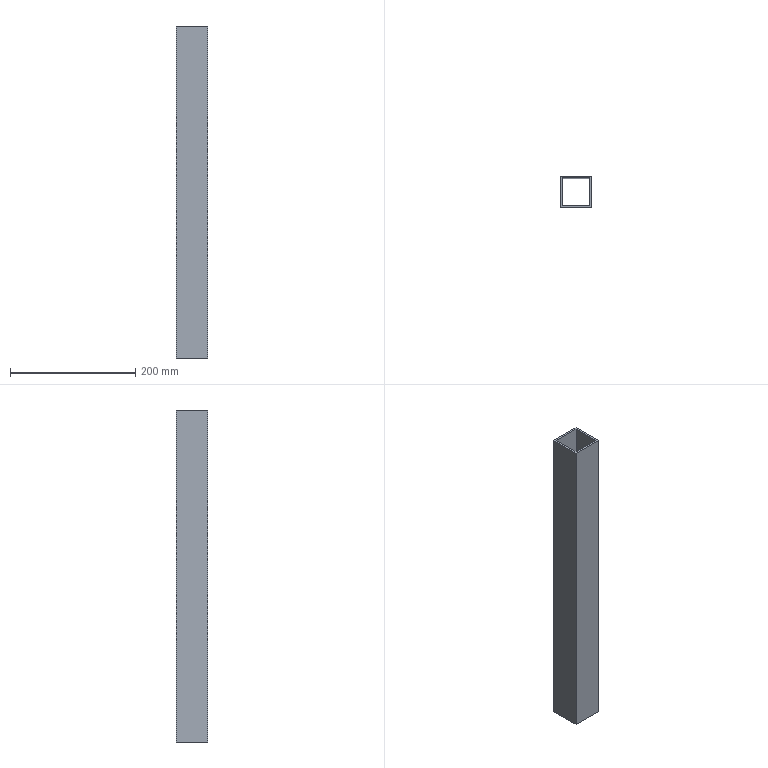Part | STEP file | BCC3 H19_4 | 1 solid | 10 faces | box 50 x 50 x 530 mm | volume 298920 mm3 | plane 10
STEP:
#1=CARTESIAN_POINT('',(0.,0.,0.));
#2=DIRECTION('',(0.,0.,1.));
#3=DIRECTION('',(1.,0.,0.));
#4=AXIS2_PLACEMENT_3D('',#1,#2,#3);
#5=CARTESIAN_POINT('',(-25.,25.,265.));
#6=VERTEX_POINT('',#5);
#7=CARTESIAN_POINT('',(-25.,-25.,265.));
#8=VERTEX_POINT('',#7);
#9=CARTESIAN_POINT('',(-25.,25.,265.));
#10=DIRECTION('',(0.,-1.,0.));
#11=VECTOR('',#10,1.);
#12=LINE('',#9,#11);
#13=CARTESIAN_POINT('',(0.,0.,265.));
#14=DIRECTION('',(0.,0.,1.));
#15=DIRECTION('',(1.,0.,0.));
#16=AXIS2_PLACEMENT_3D('',#13,#14,#15);
#17=PLANE('',#16);
#18=CARTESIAN_POINT('',(-25.,25.));
#19=DIRECTION('',(0.,-1.));
#20=VECTOR('',#19,1.);
#21=LINE('',#18,#20);
#22=(GEOMETRIC_REPRESENTATION_CONTEXT(2)PARAMETRIC_REPRESENTATION_CONTEXT()REPRESENTATION_CONTEXT('',''));
#23=DEFINITIONAL_REPRESENTATION('',(#21),#22);
#24=PCURVE('',#17,#23);
#25=CARTESIAN_POINT('',(-25.,25.,265.));
#26=DIRECTION('',(1.,0.,0.));
#27=DIRECTION('',(0.,1.,0.));
#28=AXIS2_PLACEMENT_3D('',#25,#26,#27);
#29=PLANE('',#28);
#30=CARTESIAN_POINT('',(0.,0.));
#31=DIRECTION('',(-1.,0.));
#32=VECTOR('',#31,1.);
#33=LINE('',#30,#32);
#34=(GEOMETRIC_REPRESENTATION_CONTEXT(2)PARAMETRIC_REPRESENTATION_CONTEXT()REPRESENTATION_CONTEXT('',''));
#35=DEFINITIONAL_REPRESENTATION('',(#33),#34);
#36=PCURVE('',#29,#35);
#37=SURFACE_CURVE('',#12,(#24,#36),.PCURVE_S1.);
#38=EDGE_CURVE('',#6,#8,#37,.T.);
#39=ORIENTED_EDGE('',*,*,#38,.T.);
#40=CARTESIAN_POINT('',(25.,-25.,265.));
#41=VERTEX_POINT('',#40);
#42=CARTESIAN_POINT('',(-25.,-25.,265.));
#43=DIRECTION('',(1.,0.,0.));
#44=VECTOR('',#43,1.);
#45=LINE('',#42,#44);
#46=CARTESIAN_POINT('',(-25.,-25.));
#47=DIRECTION('',(1.,0.));
#48=VECTOR('',#47,1.);
#49=LINE('',#46,#48);
#50=(GEOMETRIC_REPRESENTATION_CONTEXT(2)PARAMETRIC_REPRESENTATION_CONTEXT()REPRESENTATION_CONTEXT('',''));
#51=DEFINITIONAL_REPRESENTATION('',(#49),#50);
#52=PCURVE('',#17,#51);
#53=CARTESIAN_POINT('',(-25.,-25.,265.));
#54=DIRECTION('',(0.,1.,0.));
#55=DIRECTION('',(0.,0.,1.));
#56=AXIS2_PLACEMENT_3D('',#53,#54,#55);
#57=PLANE('',#56);
#58=CARTESIAN_POINT('',(0.,0.));
#59=DIRECTION('',(0.,1.));
#60=VECTOR('',#59,1.);
#61=LINE('',#58,#60);
#62=(GEOMETRIC_REPRESENTATION_CONTEXT(2)PARAMETRIC_REPRESENTATION_CONTEXT()REPRESENTATION_CONTEXT('',''));
#63=DEFINITIONAL_REPRESENTATION('',(#61),#62);
#64=PCURVE('',#57,#63);
#65=SURFACE_CURVE('',#45,(#52,#64),.PCURVE_S1.);
#66=EDGE_CURVE('',#8,#41,#65,.T.);
#67=ORIENTED_EDGE('',*,*,#66,.T.);
#68=CARTESIAN_POINT('',(25.,25.,265.));
#69=VERTEX_POINT('',#68);
#70=CARTESIAN_POINT('',(25.,25.,265.));
#71=DIRECTION('',(0.,1.,0.));
#72=VECTOR('',#71,1.);
#73=LINE('',#70,#72);
#74=CARTESIAN_POINT('',(25.,25.));
#75=DIRECTION('',(0.,1.));
#76=VECTOR('',#75,1.);
#77=LINE('',#74,#76);
#78=(GEOMETRIC_REPRESENTATION_CONTEXT(2)PARAMETRIC_REPRESENTATION_CONTEXT()REPRESENTATION_CONTEXT('',''));
#79=DEFINITIONAL_REPRESENTATION('',(#77),#78);
#80=PCURVE('',#17,#79);
#81=CARTESIAN_POINT('',(25.,25.,265.));
#82=DIRECTION('',(-1.,0.,0.));
#83=DIRECTION('',(0.,-1.,0.));
#84=AXIS2_PLACEMENT_3D('',#81,#82,#83);
#85=PLANE('',#84);
#86=CARTESIAN_POINT('',(0.,0.));
#87=DIRECTION('',(-1.,0.));
#88=VECTOR('',#87,1.);
#89=LINE('',#86,#88);
#90=(GEOMETRIC_REPRESENTATION_CONTEXT(2)PARAMETRIC_REPRESENTATION_CONTEXT()REPRESENTATION_CONTEXT('',''));
#91=DEFINITIONAL_REPRESENTATION('',(#89),#90);
#92=PCURVE('',#85,#91);
#93=SURFACE_CURVE('',#73,(#80,#92),.PCURVE_S1.);
#94=EDGE_CURVE('',#41,#69,#93,.T.);
#95=ORIENTED_EDGE('',*,*,#94,.T.);
#96=CARTESIAN_POINT('',(-25.,25.,265.));
#97=DIRECTION('',(-1.,0.,0.));
#98=VECTOR('',#97,1.);
#99=LINE('',#96,#98);
#100=CARTESIAN_POINT('',(-25.,25.));
#101=DIRECTION('',(-1.,0.));
#102=VECTOR('',#101,1.);
#103=LINE('',#100,#102);
#104=(GEOMETRIC_REPRESENTATION_CONTEXT(2)PARAMETRIC_REPRESENTATION_CONTEXT()REPRESENTATION_CONTEXT('',''));
#105=DEFINITIONAL_REPRESENTATION('',(#103),#104);
#106=PCURVE('',#17,#105);
#107=CARTESIAN_POINT('',(-25.,25.,265.));
#108=DIRECTION('',(0.,-1.,0.));
#109=DIRECTION('',(0.,0.,-1.));
#110=AXIS2_PLACEMENT_3D('',#107,#108,#109);
#111=PLANE('',#110);
#112=CARTESIAN_POINT('',(0.,0.));
#113=DIRECTION('',(0.,-1.));
#114=VECTOR('',#113,1.);
#115=LINE('',#112,#114);
#116=(GEOMETRIC_REPRESENTATION_CONTEXT(2)PARAMETRIC_REPRESENTATION_CONTEXT()REPRESENTATION_CONTEXT('',''));
#117=DEFINITIONAL_REPRESENTATION('',(#115),#116);
#118=PCURVE('',#111,#117);
#119=SURFACE_CURVE('',#99,(#106,#118),.PCURVE_S1.);
#120=EDGE_CURVE('',#69,#6,#119,.T.);
#121=ORIENTED_EDGE('',*,*,#120,.T.);
#122=EDGE_LOOP('',(#39,#67,#95,#121));
#123=FACE_BOUND('',#122,.T.);
#124=CARTESIAN_POINT('',(-22.,-22.,265.));
#125=VERTEX_POINT('',#124);
#126=CARTESIAN_POINT('',(22.,-22.,265.));
#127=VERTEX_POINT('',#126);
#128=CARTESIAN_POINT('',(-22.,-22.,265.));
#129=DIRECTION('',(1.,0.,0.));
#130=VECTOR('',#129,1.);
#131=LINE('',#128,#130);
#132=CARTESIAN_POINT('',(-22.,-22.));
#133=DIRECTION('',(1.,0.));
#134=VECTOR('',#133,1.);
#135=LINE('',#132,#134);
#136=(GEOMETRIC_REPRESENTATION_CONTEXT(2)PARAMETRIC_REPRESENTATION_CONTEXT()REPRESENTATION_CONTEXT('',''));
#137=DEFINITIONAL_REPRESENTATION('',(#135),#136);
#138=PCURVE('',#17,#137);
#139=CARTESIAN_POINT('',(-22.,-22.,265.));
#140=DIRECTION('',(0.,1.,0.));
#141=DIRECTION('',(-1.,0.,0.));
#142=AXIS2_PLACEMENT_3D('',#139,#140,#141);
#143=PLANE('',#142);
#144=CARTESIAN_POINT('',(0.,0.));
#145=DIRECTION('',(-1.,0.));
#146=VECTOR('',#145,1.);
#147=LINE('',#144,#146);
#148=(GEOMETRIC_REPRESENTATION_CONTEXT(2)PARAMETRIC_REPRESENTATION_CONTEXT()REPRESENTATION_CONTEXT('',''));
#149=DEFINITIONAL_REPRESENTATION('',(#147),#148);
#150=PCURVE('',#143,#149);
#151=SURFACE_CURVE('',#131,(#138,#150),.PCURVE_S1.);
#152=EDGE_CURVE('',#125,#127,#151,.T.);
#153=ORIENTED_EDGE('',*,*,#152,.F.);
#154=CARTESIAN_POINT('',(-22.,22.,265.));
#155=VERTEX_POINT('',#154);
#156=CARTESIAN_POINT('',(-22.,22.,265.));
#157=DIRECTION('',(0.,-1.,0.));
#158=VECTOR('',#157,1.);
#159=LINE('',#156,#158);
#160=CARTESIAN_POINT('',(-22.,22.));
#161=DIRECTION('',(0.,-1.));
#162=VECTOR('',#161,1.);
#163=LINE('',#160,#162);
#164=(GEOMETRIC_REPRESENTATION_CONTEXT(2)PARAMETRIC_REPRESENTATION_CONTEXT()REPRESENTATION_CONTEXT('',''));
#165=DEFINITIONAL_REPRESENTATION('',(#163),#164);
#166=PCURVE('',#17,#165);
#167=CARTESIAN_POINT('',(-22.,22.,265.));
#168=DIRECTION('',(1.,0.,0.));
#169=DIRECTION('',(0.,1.,0.));
#170=AXIS2_PLACEMENT_3D('',#167,#168,#169);
#171=PLANE('',#170);
#172=CARTESIAN_POINT('',(0.,0.));
#173=DIRECTION('',(-1.,0.));
#174=VECTOR('',#173,1.);
#175=LINE('',#172,#174);
#176=(GEOMETRIC_REPRESENTATION_CONTEXT(2)PARAMETRIC_REPRESENTATION_CONTEXT()REPRESENTATION_CONTEXT('',''));
#177=DEFINITIONAL_REPRESENTATION('',(#175),#176);
#178=PCURVE('',#171,#177);
#179=SURFACE_CURVE('',#159,(#166,#178),.PCURVE_S1.);
#180=EDGE_CURVE('',#155,#125,#179,.T.);
#181=ORIENTED_EDGE('',*,*,#180,.F.);
#182=CARTESIAN_POINT('',(22.,22.,265.));
#183=VERTEX_POINT('',#182);
#184=CARTESIAN_POINT('',(-22.,22.,265.));
#185=DIRECTION('',(-1.,0.,0.));
#186=VECTOR('',#185,1.);
#187=LINE('',#184,#186);
#188=CARTESIAN_POINT('',(-22.,22.));
#189=DIRECTION('',(-1.,0.));
#190=VECTOR('',#189,1.);
#191=LINE('',#188,#190);
#192=(GEOMETRIC_REPRESENTATION_CONTEXT(2)PARAMETRIC_REPRESENTATION_CONTEXT()REPRESENTATION_CONTEXT('',''));
#193=DEFINITIONAL_REPRESENTATION('',(#191),#192);
#194=PCURVE('',#17,#193);
#195=CARTESIAN_POINT('',(-22.,22.,265.));
#196=DIRECTION('',(0.,-1.,0.));
#197=DIRECTION('',(0.,0.,-1.));
#198=AXIS2_PLACEMENT_3D('',#195,#196,#197);
#199=PLANE('',#198);
#200=CARTESIAN_POINT('',(0.,0.));
#201=DIRECTION('',(0.,-1.));
#202=VECTOR('',#201,1.);
#203=LINE('',#200,#202);
#204=(GEOMETRIC_REPRESENTATION_CONTEXT(2)PARAMETRIC_REPRESENTATION_CONTEXT()REPRESENTATION_CONTEXT('',''));
#205=DEFINITIONAL_REPRESENTATION('',(#203),#204);
#206=PCURVE('',#199,#205);
#207=SURFACE_CURVE('',#187,(#194,#206),.PCURVE_S1.);
#208=EDGE_CURVE('',#183,#155,#207,.T.);
#209=ORIENTED_EDGE('',*,*,#208,.F.);
#210=CARTESIAN_POINT('',(22.,22.,265.));
#211=DIRECTION('',(0.,1.,0.));
#212=VECTOR('',#211,1.);
#213=LINE('',#210,#212);
#214=CARTESIAN_POINT('',(22.,22.));
#215=DIRECTION('',(0.,1.));
#216=VECTOR('',#215,1.);
#217=LINE('',#214,#216);
#218=(GEOMETRIC_REPRESENTATION_CONTEXT(2)PARAMETRIC_REPRESENTATION_CONTEXT()REPRESENTATION_CONTEXT('',''));
#219=DEFINITIONAL_REPRESENTATION('',(#217),#218);
#220=PCURVE('',#17,#219);
#221=CARTESIAN_POINT('',(22.,22.,265.));
#222=DIRECTION('',(-1.,0.,0.));
#223=DIRECTION('',(0.,-1.,0.));
#224=AXIS2_PLACEMENT_3D('',#221,#222,#223);
#225=PLANE('',#224);
#226=CARTESIAN_POINT('',(0.,0.));
#227=DIRECTION('',(-1.,0.));
#228=VECTOR('',#227,1.);
#229=LINE('',#226,#228);
#230=(GEOMETRIC_REPRESENTATION_CONTEXT(2)PARAMETRIC_REPRESENTATION_CONTEXT()REPRESENTATION_CONTEXT('',''));
#231=DEFINITIONAL_REPRESENTATION('',(#229),#230);
#232=PCURVE('',#225,#231);
#233=SURFACE_CURVE('',#213,(#220,#232),.PCURVE_S1.);
#234=EDGE_CURVE('',#127,#183,#233,.T.);
#235=ORIENTED_EDGE('',*,*,#234,.F.);
#236=EDGE_LOOP('',(#153,#181,#209,#235));
#237=FACE_BOUND('',#236,.T.);
#238=ADVANCED_FACE('',(#123,#237),#17,.T.);
#239=CARTESIAN_POINT('',(-25.,25.,-265.));
#240=VERTEX_POINT('',#239);
#241=CARTESIAN_POINT('',(-25.,-25.,-265.));
#242=VERTEX_POINT('',#241);
#243=CARTESIAN_POINT('',(-25.,25.,-265.));
#244=DIRECTION('',(0.,-1.,0.));
#245=VECTOR('',#244,1.);
#246=LINE('',#243,#245);
#247=CARTESIAN_POINT('',(0.,0.,-265.));
#248=DIRECTION('',(0.,0.,1.));
#249=DIRECTION('',(1.,0.,0.));
#250=AXIS2_PLACEMENT_3D('',#247,#248,#249);
#251=PLANE('',#250);
#252=CARTESIAN_POINT('',(-25.,25.));
#253=DIRECTION('',(0.,-1.));
#254=VECTOR('',#253,1.);
#255=LINE('',#252,#254);
#256=(GEOMETRIC_REPRESENTATION_CONTEXT(2)PARAMETRIC_REPRESENTATION_CONTEXT()REPRESENTATION_CONTEXT('',''));
#257=DEFINITIONAL_REPRESENTATION('',(#255),#256);
#258=PCURVE('',#251,#257);
#259=CARTESIAN_POINT('',(0.,-530.));
#260=DIRECTION('',(-1.,0.));
#261=VECTOR('',#260,1.);
#262=LINE('',#259,#261);
#263=(GEOMETRIC_REPRESENTATION_CONTEXT(2)PARAMETRIC_REPRESENTATION_CONTEXT()REPRESENTATION_CONTEXT('',''));
#264=DEFINITIONAL_REPRESENTATION('',(#262),#263);
#265=PCURVE('',#29,#264);
#266=SURFACE_CURVE('',#246,(#258,#265),.PCURVE_S1.);
#267=EDGE_CURVE('',#240,#242,#266,.T.);
#268=ORIENTED_EDGE('',*,*,#267,.F.);
#269=CARTESIAN_POINT('',(25.,25.,-265.));
#270=VERTEX_POINT('',#269);
#271=CARTESIAN_POINT('',(-25.,25.,-265.));
#272=DIRECTION('',(-1.,0.,0.));
#273=VECTOR('',#272,1.);
#274=LINE('',#271,#273);
#275=CARTESIAN_POINT('',(-25.,25.));
#276=DIRECTION('',(-1.,0.));
#277=VECTOR('',#276,1.);
#278=LINE('',#275,#277);
#279=(GEOMETRIC_REPRESENTATION_CONTEXT(2)PARAMETRIC_REPRESENTATION_CONTEXT()REPRESENTATION_CONTEXT('',''));
#280=DEFINITIONAL_REPRESENTATION('',(#278),#279);
#281=PCURVE('',#251,#280);
#282=CARTESIAN_POINT('',(530.,0.));
#283=DIRECTION('',(0.,-1.));
#284=VECTOR('',#283,1.);
#285=LINE('',#282,#284);
#286=(GEOMETRIC_REPRESENTATION_CONTEXT(2)PARAMETRIC_REPRESENTATION_CONTEXT()REPRESENTATION_CONTEXT('',''));
#287=DEFINITIONAL_REPRESENTATION('',(#285),#286);
#288=PCURVE('',#111,#287);
#289=SURFACE_CURVE('',#274,(#281,#288),.PCURVE_S1.);
#290=EDGE_CURVE('',#270,#240,#289,.T.);
#291=ORIENTED_EDGE('',*,*,#290,.F.);
#292=CARTESIAN_POINT('',(25.,-25.,-265.));
#293=VERTEX_POINT('',#292);
#294=CARTESIAN_POINT('',(25.,25.,-265.));
#295=DIRECTION('',(0.,1.,0.));
#296=VECTOR('',#295,1.);
#297=LINE('',#294,#296);
#298=CARTESIAN_POINT('',(25.,25.));
#299=DIRECTION('',(0.,1.));
#300=VECTOR('',#299,1.);
#301=LINE('',#298,#300);
#302=(GEOMETRIC_REPRESENTATION_CONTEXT(2)PARAMETRIC_REPRESENTATION_CONTEXT()REPRESENTATION_CONTEXT('',''));
#303=DEFINITIONAL_REPRESENTATION('',(#301),#302);
#304=PCURVE('',#251,#303);
#305=CARTESIAN_POINT('',(0.,-530.));
#306=DIRECTION('',(-1.,0.));
#307=VECTOR('',#306,1.);
#308=LINE('',#305,#307);
#309=(GEOMETRIC_REPRESENTATION_CONTEXT(2)PARAMETRIC_REPRESENTATION_CONTEXT()REPRESENTATION_CONTEXT('',''));
#310=DEFINITIONAL_REPRESENTATION('',(#308),#309);
#311=PCURVE('',#85,#310);
#312=SURFACE_CURVE('',#297,(#304,#311),.PCURVE_S1.);
#313=EDGE_CURVE('',#293,#270,#312,.T.);
#314=ORIENTED_EDGE('',*,*,#313,.F.);
#315=CARTESIAN_POINT('',(-25.,-25.,-265.));
#316=DIRECTION('',(1.,0.,0.));
#317=VECTOR('',#316,1.);
#318=LINE('',#315,#317);
#319=CARTESIAN_POINT('',(-25.,-25.));
#320=DIRECTION('',(1.,0.));
#321=VECTOR('',#320,1.);
#322=LINE('',#319,#321);
#323=(GEOMETRIC_REPRESENTATION_CONTEXT(2)PARAMETRIC_REPRESENTATION_CONTEXT()REPRESENTATION_CONTEXT('',''));
#324=DEFINITIONAL_REPRESENTATION('',(#322),#323);
#325=PCURVE('',#251,#324);
#326=CARTESIAN_POINT('',(-530.,0.));
#327=DIRECTION('',(0.,1.));
#328=VECTOR('',#327,1.);
#329=LINE('',#326,#328);
#330=(GEOMETRIC_REPRESENTATION_CONTEXT(2)PARAMETRIC_REPRESENTATION_CONTEXT()REPRESENTATION_CONTEXT('',''));
#331=DEFINITIONAL_REPRESENTATION('',(#329),#330);
#332=PCURVE('',#57,#331);
#333=SURFACE_CURVE('',#318,(#325,#332),.PCURVE_S1.);
#334=EDGE_CURVE('',#242,#293,#333,.T.);
#335=ORIENTED_EDGE('',*,*,#334,.F.);
#336=EDGE_LOOP('',(#268,#291,#314,#335));
#337=FACE_BOUND('',#336,.T.);
#338=CARTESIAN_POINT('',(-22.,22.,-265.));
#339=VERTEX_POINT('',#338);
#340=CARTESIAN_POINT('',(-22.,-22.,-265.));
#341=VERTEX_POINT('',#340);
#342=CARTESIAN_POINT('',(-22.,22.,-265.));
#343=DIRECTION('',(0.,-1.,0.));
#344=VECTOR('',#343,1.);
#345=LINE('',#342,#344);
#346=CARTESIAN_POINT('',(-22.,22.));
#347=DIRECTION('',(0.,-1.));
#348=VECTOR('',#347,1.);
#349=LINE('',#346,#348);
#350=(GEOMETRIC_REPRESENTATION_CONTEXT(2)PARAMETRIC_REPRESENTATION_CONTEXT()REPRESENTATION_CONTEXT('',''));
#351=DEFINITIONAL_REPRESENTATION('',(#349),#350);
#352=PCURVE('',#251,#351);
#353=CARTESIAN_POINT('',(0.,-530.));
#354=DIRECTION('',(-1.,0.));
#355=VECTOR('',#354,1.);
#356=LINE('',#353,#355);
#357=(GEOMETRIC_REPRESENTATION_CONTEXT(2)PARAMETRIC_REPRESENTATION_CONTEXT()REPRESENTATION_CONTEXT('',''));
#358=DEFINITIONAL_REPRESENTATION('',(#356),#357);
#359=PCURVE('',#171,#358);
#360=SURFACE_CURVE('',#345,(#352,#359),.PCURVE_S1.);
#361=EDGE_CURVE('',#339,#341,#360,.T.);
#362=ORIENTED_EDGE('',*,*,#361,.T.);
#363=CARTESIAN_POINT('',(22.,-22.,-265.));
#364=VERTEX_POINT('',#363);
#365=CARTESIAN_POINT('',(-22.,-22.,-265.));
#366=DIRECTION('',(1.,0.,0.));
#367=VECTOR('',#366,1.);
#368=LINE('',#365,#367);
#369=CARTESIAN_POINT('',(-22.,-22.));
#370=DIRECTION('',(1.,0.));
#371=VECTOR('',#370,1.);
#372=LINE('',#369,#371);
#373=(GEOMETRIC_REPRESENTATION_CONTEXT(2)PARAMETRIC_REPRESENTATION_CONTEXT()REPRESENTATION_CONTEXT('',''));
#374=DEFINITIONAL_REPRESENTATION('',(#372),#373);
#375=PCURVE('',#251,#374);
#376=CARTESIAN_POINT('',(0.,-530.));
#377=DIRECTION('',(-1.,0.));
#378=VECTOR('',#377,1.);
#379=LINE('',#376,#378);
#380=(GEOMETRIC_REPRESENTATION_CONTEXT(2)PARAMETRIC_REPRESENTATION_CONTEXT()REPRESENTATION_CONTEXT('',''));
#381=DEFINITIONAL_REPRESENTATION('',(#379),#380);
#382=PCURVE('',#143,#381);
#383=SURFACE_CURVE('',#368,(#375,#382),.PCURVE_S1.);
#384=EDGE_CURVE('',#341,#364,#383,.T.);
#385=ORIENTED_EDGE('',*,*,#384,.T.);
#386=CARTESIAN_POINT('',(22.,22.,-265.));
#387=VERTEX_POINT('',#386);
#388=CARTESIAN_POINT('',(22.,22.,-265.));
#389=DIRECTION('',(0.,1.,0.));
#390=VECTOR('',#389,1.);
#391=LINE('',#388,#390);
#392=CARTESIAN_POINT('',(22.,22.));
#393=DIRECTION('',(0.,1.));
#394=VECTOR('',#393,1.);
#395=LINE('',#392,#394);
#396=(GEOMETRIC_REPRESENTATION_CONTEXT(2)PARAMETRIC_REPRESENTATION_CONTEXT()REPRESENTATION_CONTEXT('',''));
#397=DEFINITIONAL_REPRESENTATION('',(#395),#396);
#398=PCURVE('',#251,#397);
#399=CARTESIAN_POINT('',(0.,-530.));
#400=DIRECTION('',(-1.,0.));
#401=VECTOR('',#400,1.);
#402=LINE('',#399,#401);
#403=(GEOMETRIC_REPRESENTATION_CONTEXT(2)PARAMETRIC_REPRESENTATION_CONTEXT()REPRESENTATION_CONTEXT('',''));
#404=DEFINITIONAL_REPRESENTATION('',(#402),#403);
#405=PCURVE('',#225,#404);
#406=SURFACE_CURVE('',#391,(#398,#405),.PCURVE_S1.);
#407=EDGE_CURVE('',#364,#387,#406,.T.);
#408=ORIENTED_EDGE('',*,*,#407,.T.);
#409=CARTESIAN_POINT('',(-22.,22.,-265.));
#410=DIRECTION('',(-1.,0.,0.));
#411=VECTOR('',#410,1.);
#412=LINE('',#409,#411);
#413=CARTESIAN_POINT('',(-22.,22.));
#414=DIRECTION('',(-1.,0.));
#415=VECTOR('',#414,1.);
#416=LINE('',#413,#415);
#417=(GEOMETRIC_REPRESENTATION_CONTEXT(2)PARAMETRIC_REPRESENTATION_CONTEXT()REPRESENTATION_CONTEXT('',''));
#418=DEFINITIONAL_REPRESENTATION('',(#416),#417);
#419=PCURVE('',#251,#418);
#420=CARTESIAN_POINT('',(530.,0.));
#421=DIRECTION('',(0.,-1.));
#422=VECTOR('',#421,1.);
#423=LINE('',#420,#422);
#424=(GEOMETRIC_REPRESENTATION_CONTEXT(2)PARAMETRIC_REPRESENTATION_CONTEXT()REPRESENTATION_CONTEXT('',''));
#425=DEFINITIONAL_REPRESENTATION('',(#423),#424);
#426=PCURVE('',#199,#425);
#427=SURFACE_CURVE('',#412,(#419,#426),.PCURVE_S1.);
#428=EDGE_CURVE('',#387,#339,#427,.T.);
#429=ORIENTED_EDGE('',*,*,#428,.T.);
#430=EDGE_LOOP('',(#362,#385,#408,#429));
#431=FACE_BOUND('',#430,.T.);
#432=ADVANCED_FACE('',(#337,#431),#251,.F.);
#433=ORIENTED_EDGE('',*,*,#267,.T.);
#434=CARTESIAN_POINT('',(-25.,-25.,265.));
#435=DIRECTION('',(0.,0.,-1.));
#436=VECTOR('',#435,1.);
#437=LINE('',#434,#436);
#438=CARTESIAN_POINT('',(-50.,0.));
#439=DIRECTION('',(0.,-1.));
#440=VECTOR('',#439,1.);
#441=LINE('',#438,#440);
#442=(GEOMETRIC_REPRESENTATION_CONTEXT(2)PARAMETRIC_REPRESENTATION_CONTEXT()REPRESENTATION_CONTEXT('',''));
#443=DEFINITIONAL_REPRESENTATION('',(#441),#442);
#444=PCURVE('',#29,#443);
#445=CARTESIAN_POINT('',(0.,0.));
#446=DIRECTION('',(-1.,0.));
#447=VECTOR('',#446,1.);
#448=LINE('',#445,#447);
#449=(GEOMETRIC_REPRESENTATION_CONTEXT(2)PARAMETRIC_REPRESENTATION_CONTEXT()REPRESENTATION_CONTEXT('',''));
#450=DEFINITIONAL_REPRESENTATION('',(#448),#449);
#451=PCURVE('',#57,#450);
#452=SURFACE_CURVE('',#437,(#444,#451),.PCURVE_S1.);
#453=EDGE_CURVE('',#8,#242,#452,.T.);
#454=ORIENTED_EDGE('',*,*,#453,.F.);
#455=ORIENTED_EDGE('',*,*,#38,.F.);
#456=CARTESIAN_POINT('',(-25.,25.,265.));
#457=DIRECTION('',(0.,0.,-1.));
#458=VECTOR('',#457,1.);
#459=LINE('',#456,#458);
#460=CARTESIAN_POINT('',(0.,0.));
#461=DIRECTION('',(0.,-1.));
#462=VECTOR('',#461,1.);
#463=LINE('',#460,#462);
#464=(GEOMETRIC_REPRESENTATION_CONTEXT(2)PARAMETRIC_REPRESENTATION_CONTEXT()REPRESENTATION_CONTEXT('',''));
#465=DEFINITIONAL_REPRESENTATION('',(#463),#464);
#466=PCURVE('',#29,#465);
#467=CARTESIAN_POINT('',(0.,0.));
#468=DIRECTION('',(1.,0.));
#469=VECTOR('',#468,1.);
#470=LINE('',#467,#469);
#471=(GEOMETRIC_REPRESENTATION_CONTEXT(2)PARAMETRIC_REPRESENTATION_CONTEXT()REPRESENTATION_CONTEXT('',''));
#472=DEFINITIONAL_REPRESENTATION('',(#470),#471);
#473=PCURVE('',#111,#472);
#474=SURFACE_CURVE('',#459,(#466,#473),.PCURVE_S1.);
#475=EDGE_CURVE('',#6,#240,#474,.T.);
#476=ORIENTED_EDGE('',*,*,#475,.T.);
#477=EDGE_LOOP('',(#433,#454,#455,#476));
#478=FACE_BOUND('',#477,.T.);
#479=ADVANCED_FACE('',(#478),#29,.F.);
#480=ORIENTED_EDGE('',*,*,#334,.T.);
#481=CARTESIAN_POINT('',(25.,-25.,265.));
#482=DIRECTION('',(0.,0.,-1.));
#483=VECTOR('',#482,1.);
#484=LINE('',#481,#483);
#485=CARTESIAN_POINT('',(0.,50.));
#486=DIRECTION('',(-1.,0.));
#487=VECTOR('',#486,1.);
#488=LINE('',#485,#487);
#489=(GEOMETRIC_REPRESENTATION_CONTEXT(2)PARAMETRIC_REPRESENTATION_CONTEXT()REPRESENTATION_CONTEXT('',''));
#490=DEFINITIONAL_REPRESENTATION('',(#488),#489);
#491=PCURVE('',#57,#490);
#492=CARTESIAN_POINT('',(50.,0.));
#493=DIRECTION('',(0.,-1.));
#494=VECTOR('',#493,1.);
#495=LINE('',#492,#494);
#496=(GEOMETRIC_REPRESENTATION_CONTEXT(2)PARAMETRIC_REPRESENTATION_CONTEXT()REPRESENTATION_CONTEXT('',''));
#497=DEFINITIONAL_REPRESENTATION('',(#495),#496);
#498=PCURVE('',#85,#497);
#499=SURFACE_CURVE('',#484,(#491,#498),.PCURVE_S1.);
#500=EDGE_CURVE('',#41,#293,#499,.T.);
#501=ORIENTED_EDGE('',*,*,#500,.F.);
#502=ORIENTED_EDGE('',*,*,#66,.F.);
#503=ORIENTED_EDGE('',*,*,#453,.T.);
#504=EDGE_LOOP('',(#480,#501,#502,#503));
#505=FACE_BOUND('',#504,.T.);
#506=ADVANCED_FACE('',(#505),#57,.F.);
#507=ORIENTED_EDGE('',*,*,#313,.T.);
#508=CARTESIAN_POINT('',(25.,25.,265.));
#509=DIRECTION('',(0.,0.,-1.));
#510=VECTOR('',#509,1.);
#511=LINE('',#508,#510);
#512=CARTESIAN_POINT('',(0.,0.));
#513=DIRECTION('',(0.,-1.));
#514=VECTOR('',#513,1.);
#515=LINE('',#512,#514);
#516=(GEOMETRIC_REPRESENTATION_CONTEXT(2)PARAMETRIC_REPRESENTATION_CONTEXT()REPRESENTATION_CONTEXT('',''));
#517=DEFINITIONAL_REPRESENTATION('',(#515),#516);
#518=PCURVE('',#85,#517);
#519=CARTESIAN_POINT('',(0.,50.));
#520=DIRECTION('',(1.,0.));
#521=VECTOR('',#520,1.);
#522=LINE('',#519,#521);
#523=(GEOMETRIC_REPRESENTATION_CONTEXT(2)PARAMETRIC_REPRESENTATION_CONTEXT()REPRESENTATION_CONTEXT('',''));
#524=DEFINITIONAL_REPRESENTATION('',(#522),#523);
#525=PCURVE('',#111,#524);
#526=SURFACE_CURVE('',#511,(#518,#525),.PCURVE_S1.);
#527=EDGE_CURVE('',#69,#270,#526,.T.);
#528=ORIENTED_EDGE('',*,*,#527,.F.);
#529=ORIENTED_EDGE('',*,*,#94,.F.);
#530=ORIENTED_EDGE('',*,*,#500,.T.);
#531=EDGE_LOOP('',(#507,#528,#529,#530));
#532=FACE_BOUND('',#531,.T.);
#533=ADVANCED_FACE('',(#532),#85,.F.);
#534=ORIENTED_EDGE('',*,*,#290,.T.);
#535=ORIENTED_EDGE('',*,*,#475,.F.);
#536=ORIENTED_EDGE('',*,*,#120,.F.);
#537=ORIENTED_EDGE('',*,*,#527,.T.);
#538=EDGE_LOOP('',(#534,#535,#536,#537));
#539=FACE_BOUND('',#538,.T.);
#540=ADVANCED_FACE('',(#539),#111,.F.);
#541=ORIENTED_EDGE('',*,*,#361,.F.);
#542=CARTESIAN_POINT('',(-22.,22.,265.));
#543=DIRECTION('',(0.,0.,-1.));
#544=VECTOR('',#543,1.);
#545=LINE('',#542,#544);
#546=CARTESIAN_POINT('',(0.,0.));
#547=DIRECTION('',(0.,-1.));
#548=VECTOR('',#547,1.);
#549=LINE('',#546,#548);
#550=(GEOMETRIC_REPRESENTATION_CONTEXT(2)PARAMETRIC_REPRESENTATION_CONTEXT()REPRESENTATION_CONTEXT('',''));
#551=DEFINITIONAL_REPRESENTATION('',(#549),#550);
#552=PCURVE('',#171,#551);
#553=CARTESIAN_POINT('',(0.,0.));
#554=DIRECTION('',(1.,0.));
#555=VECTOR('',#554,1.);
#556=LINE('',#553,#555);
#557=(GEOMETRIC_REPRESENTATION_CONTEXT(2)PARAMETRIC_REPRESENTATION_CONTEXT()REPRESENTATION_CONTEXT('',''));
#558=DEFINITIONAL_REPRESENTATION('',(#556),#557);
#559=PCURVE('',#199,#558);
#560=SURFACE_CURVE('',#545,(#552,#559),.PCURVE_S1.);
#561=EDGE_CURVE('',#155,#339,#560,.T.);
#562=ORIENTED_EDGE('',*,*,#561,.F.);
#563=ORIENTED_EDGE('',*,*,#180,.T.);
#564=CARTESIAN_POINT('',(-22.,-22.,265.));
#565=DIRECTION('',(0.,0.,-1.));
#566=VECTOR('',#565,1.);
#567=LINE('',#564,#566);
#568=CARTESIAN_POINT('',(-44.,0.));
#569=DIRECTION('',(0.,-1.));
#570=VECTOR('',#569,1.);
#571=LINE('',#568,#570);
#572=(GEOMETRIC_REPRESENTATION_CONTEXT(2)PARAMETRIC_REPRESENTATION_CONTEXT()REPRESENTATION_CONTEXT('',''));
#573=DEFINITIONAL_REPRESENTATION('',(#571),#572);
#574=PCURVE('',#171,#573);
#575=CARTESIAN_POINT('',(0.,0.));
#576=DIRECTION('',(0.,-1.));
#577=VECTOR('',#576,1.);
#578=LINE('',#575,#577);
#579=(GEOMETRIC_REPRESENTATION_CONTEXT(2)PARAMETRIC_REPRESENTATION_CONTEXT()REPRESENTATION_CONTEXT('',''));
#580=DEFINITIONAL_REPRESENTATION('',(#578),#579);
#581=PCURVE('',#143,#580);
#582=SURFACE_CURVE('',#567,(#574,#581),.PCURVE_S1.);
#583=EDGE_CURVE('',#125,#341,#582,.T.);
#584=ORIENTED_EDGE('',*,*,#583,.T.);
#585=EDGE_LOOP('',(#541,#562,#563,#584));
#586=FACE_BOUND('',#585,.T.);
#587=ADVANCED_FACE('',(#586),#171,.T.);
#588=ORIENTED_EDGE('',*,*,#384,.F.);
#589=ORIENTED_EDGE('',*,*,#583,.F.);
#590=ORIENTED_EDGE('',*,*,#152,.T.);
#591=CARTESIAN_POINT('',(22.,-22.,265.));
#592=DIRECTION('',(0.,0.,-1.));
#593=VECTOR('',#592,1.);
#594=LINE('',#591,#593);
#595=CARTESIAN_POINT('',(-44.,0.));
#596=DIRECTION('',(0.,-1.));
#597=VECTOR('',#596,1.);
#598=LINE('',#595,#597);
#599=(GEOMETRIC_REPRESENTATION_CONTEXT(2)PARAMETRIC_REPRESENTATION_CONTEXT()REPRESENTATION_CONTEXT('',''));
#600=DEFINITIONAL_REPRESENTATION('',(#598),#599);
#601=PCURVE('',#143,#600);
#602=CARTESIAN_POINT('',(44.,0.));
#603=DIRECTION('',(0.,-1.));
#604=VECTOR('',#603,1.);
#605=LINE('',#602,#604);
#606=(GEOMETRIC_REPRESENTATION_CONTEXT(2)PARAMETRIC_REPRESENTATION_CONTEXT()REPRESENTATION_CONTEXT('',''));
#607=DEFINITIONAL_REPRESENTATION('',(#605),#606);
#608=PCURVE('',#225,#607);
#609=SURFACE_CURVE('',#594,(#601,#608),.PCURVE_S1.);
#610=EDGE_CURVE('',#127,#364,#609,.T.);
#611=ORIENTED_EDGE('',*,*,#610,.T.);
#612=EDGE_LOOP('',(#588,#589,#590,#611));
#613=FACE_BOUND('',#612,.T.);
#614=ADVANCED_FACE('',(#613),#143,.T.);
#615=ORIENTED_EDGE('',*,*,#407,.F.);
#616=ORIENTED_EDGE('',*,*,#610,.F.);
#617=ORIENTED_EDGE('',*,*,#234,.T.);
#618=CARTESIAN_POINT('',(22.,22.,265.));
#619=DIRECTION('',(0.,0.,-1.));
#620=VECTOR('',#619,1.);
#621=LINE('',#618,#620);
#622=CARTESIAN_POINT('',(0.,0.));
#623=DIRECTION('',(0.,-1.));
#624=VECTOR('',#623,1.);
#625=LINE('',#622,#624);
#626=(GEOMETRIC_REPRESENTATION_CONTEXT(2)PARAMETRIC_REPRESENTATION_CONTEXT()REPRESENTATION_CONTEXT('',''));
#627=DEFINITIONAL_REPRESENTATION('',(#625),#626);
#628=PCURVE('',#225,#627);
#629=CARTESIAN_POINT('',(0.,44.));
#630=DIRECTION('',(1.,0.));
#631=VECTOR('',#630,1.);
#632=LINE('',#629,#631);
#633=(GEOMETRIC_REPRESENTATION_CONTEXT(2)PARAMETRIC_REPRESENTATION_CONTEXT()REPRESENTATION_CONTEXT('',''));
#634=DEFINITIONAL_REPRESENTATION('',(#632),#633);
#635=PCURVE('',#199,#634);
#636=SURFACE_CURVE('',#621,(#628,#635),.PCURVE_S1.);
#637=EDGE_CURVE('',#183,#387,#636,.T.);
#638=ORIENTED_EDGE('',*,*,#637,.T.);
#639=EDGE_LOOP('',(#615,#616,#617,#638));
#640=FACE_BOUND('',#639,.T.);
#641=ADVANCED_FACE('',(#640),#225,.T.);
#642=ORIENTED_EDGE('',*,*,#428,.F.);
#643=ORIENTED_EDGE('',*,*,#637,.F.);
#644=ORIENTED_EDGE('',*,*,#208,.T.);
#645=ORIENTED_EDGE('',*,*,#561,.T.);
#646=EDGE_LOOP('',(#642,#643,#644,#645));
#647=FACE_BOUND('',#646,.T.);
#648=ADVANCED_FACE('',(#647),#199,.T.);
#649=CLOSED_SHELL('',(#238,#432,#479,#506,#533,#540,#587,#614,#641,#648));
#650=MANIFOLD_SOLID_BREP('',#649);
#651=(LENGTH_UNIT()NAMED_UNIT(*)SI_UNIT(.MILLI.,.METRE.));
#652=UNCERTAINTY_MEASURE_WITH_UNIT(LENGTH_MEASURE(0.0000001),#651,'','');
#653=(NAMED_UNIT(*)PLANE_ANGLE_UNIT()SI_UNIT($,.RADIAN.));
#654=(NAMED_UNIT(*)SI_UNIT($,.STERADIAN.)SOLID_ANGLE_UNIT());
#655=(GEOMETRIC_REPRESENTATION_CONTEXT(3)GLOBAL_UNCERTAINTY_ASSIGNED_CONTEXT((#652))GLOBAL_UNIT_ASSIGNED_CONTEXT((#651,#653,#654))REPRESENTATION_CONTEXT('',''));
#656=ADVANCED_BREP_SHAPE_REPRESENTATION('',(#4,#650),#655);